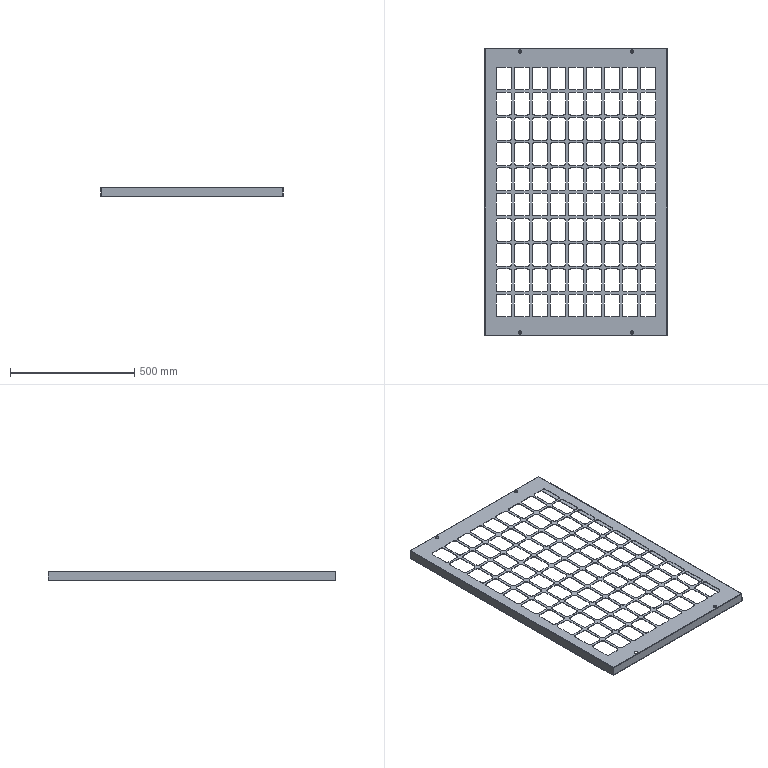Part | STEP file | SX-018-01 | 1 solid | 806 faces | box 733.501 x 1156 x 39 mm | volume 1117347 mm3 | plane 402 | cylinder 392 | spline 12 | commonest cylinder face diameters 20 x360 0.4 x8 4.4 x8 8 x8 14 x8